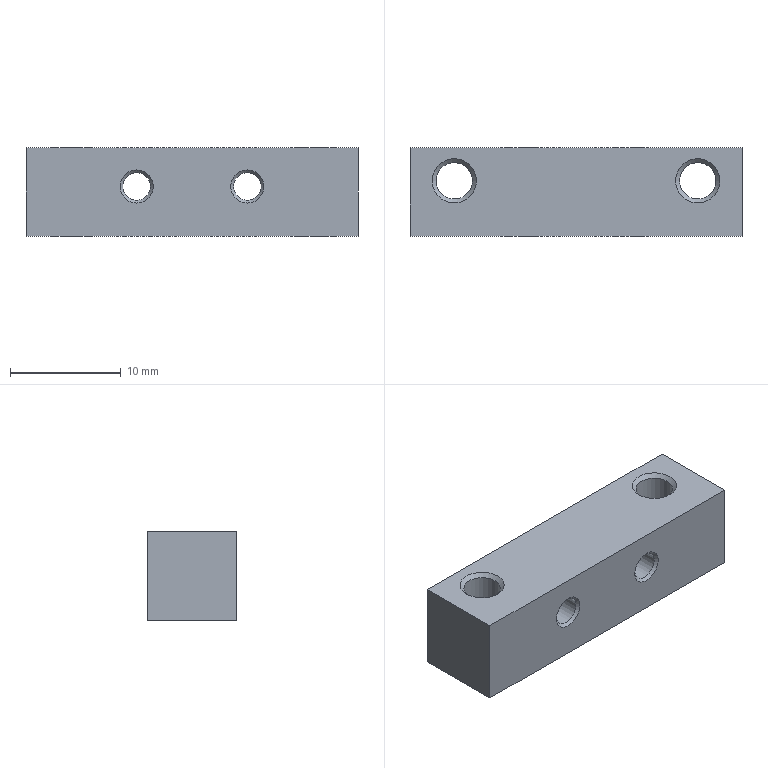Part | STEP file | Connector mounting block | 1 solid | 18 faces | box 30 x 8 x 8 mm | volume 1701 mm3 | cone 8 | plane 6 | cylinder 4 | commonest cylinder face diameters 2.5 x2 3.3 x2
STEP:
#1=CARTESIAN_POINT('',(0.,0.,0.));
#2=DIRECTION('',(0.,0.,1.));
#3=DIRECTION('',(1.,0.,0.));
#4=AXIS2_PLACEMENT_3D('',#1,#2,#3);
#5=CARTESIAN_POINT('',(-15.,4.,0.));
#6=VERTEX_POINT('',#5);
#7=CARTESIAN_POINT('',(-15.,-4.,0.));
#8=VERTEX_POINT('',#7);
#9=CARTESIAN_POINT('',(-15.,4.,0.));
#10=DIRECTION('',(0.,-1.,0.));
#11=VECTOR('',#10,1.);
#12=LINE('',#9,#11);
#13=CARTESIAN_POINT('',(-15.,4.,4.));
#14=DIRECTION('',(1.,0.,0.));
#15=DIRECTION('',(0.,1.,0.));
#16=AXIS2_PLACEMENT_3D('',#13,#14,#15);
#17=PLANE('',#16);
#18=CARTESIAN_POINT('',(0.,-4.));
#19=DIRECTION('',(-1.,0.));
#20=VECTOR('',#19,1.);
#21=LINE('',#18,#20);
#22=(GEOMETRIC_REPRESENTATION_CONTEXT(2)PARAMETRIC_REPRESENTATION_CONTEXT()REPRESENTATION_CONTEXT('',''));
#23=DEFINITIONAL_REPRESENTATION('',(#21),#22);
#24=PCURVE('',#17,#23);
#25=CARTESIAN_POINT('',(0.,0.,0.));
#26=DIRECTION('',(0.,0.,1.));
#27=DIRECTION('',(1.,0.,0.));
#28=AXIS2_PLACEMENT_3D('',#25,#26,#27);
#29=PLANE('',#28);
#30=CARTESIAN_POINT('',(-15.,4.));
#31=DIRECTION('',(0.,-1.));
#32=VECTOR('',#31,1.);
#33=LINE('',#30,#32);
#34=(GEOMETRIC_REPRESENTATION_CONTEXT(2)PARAMETRIC_REPRESENTATION_CONTEXT()REPRESENTATION_CONTEXT('',''));
#35=DEFINITIONAL_REPRESENTATION('',(#33),#34);
#36=PCURVE('',#29,#35);
#37=SURFACE_CURVE('',#12,(#24,#36),.PCURVE_S1.);
#38=EDGE_CURVE('',#6,#8,#37,.T.);
#39=ORIENTED_EDGE('',*,*,#38,.T.);
#40=CARTESIAN_POINT('',(-15.,-4.,8.));
#41=VERTEX_POINT('',#40);
#42=CARTESIAN_POINT('',(-15.,-4.,4.));
#43=DIRECTION('',(0.,0.,-1.));
#44=VECTOR('',#43,1.);
#45=LINE('',#42,#44);
#46=CARTESIAN_POINT('',(-8.,0.));
#47=DIRECTION('',(0.,-1.));
#48=VECTOR('',#47,1.);
#49=LINE('',#46,#48);
#50=(GEOMETRIC_REPRESENTATION_CONTEXT(2)PARAMETRIC_REPRESENTATION_CONTEXT()REPRESENTATION_CONTEXT('',''));
#51=DEFINITIONAL_REPRESENTATION('',(#49),#50);
#52=PCURVE('',#17,#51);
#53=CARTESIAN_POINT('',(-15.,-4.,4.));
#54=DIRECTION('',(0.,1.,0.));
#55=DIRECTION('',(0.,0.,1.));
#56=AXIS2_PLACEMENT_3D('',#53,#54,#55);
#57=PLANE('',#56);
#58=CARTESIAN_POINT('',(0.,0.));
#59=DIRECTION('',(-1.,0.));
#60=VECTOR('',#59,1.);
#61=LINE('',#58,#60);
#62=(GEOMETRIC_REPRESENTATION_CONTEXT(2)PARAMETRIC_REPRESENTATION_CONTEXT()REPRESENTATION_CONTEXT('',''));
#63=DEFINITIONAL_REPRESENTATION('',(#61),#62);
#64=PCURVE('',#57,#63);
#65=SURFACE_CURVE('',#45,(#52,#64),.PCURVE_S1.);
#66=EDGE_CURVE('',#41,#8,#65,.T.);
#67=ORIENTED_EDGE('',*,*,#66,.F.);
#68=CARTESIAN_POINT('',(-15.,4.,8.));
#69=VERTEX_POINT('',#68);
#70=CARTESIAN_POINT('',(-15.,4.,8.));
#71=DIRECTION('',(0.,-1.,0.));
#72=VECTOR('',#71,1.);
#73=LINE('',#70,#72);
#74=CARTESIAN_POINT('',(0.,4.));
#75=DIRECTION('',(-1.,0.));
#76=VECTOR('',#75,1.);
#77=LINE('',#74,#76);
#78=(GEOMETRIC_REPRESENTATION_CONTEXT(2)PARAMETRIC_REPRESENTATION_CONTEXT()REPRESENTATION_CONTEXT('',''));
#79=DEFINITIONAL_REPRESENTATION('',(#77),#78);
#80=PCURVE('',#17,#79);
#81=CARTESIAN_POINT('',(0.,0.,8.));
#82=DIRECTION('',(0.,0.,1.));
#83=DIRECTION('',(1.,0.,0.));
#84=AXIS2_PLACEMENT_3D('',#81,#82,#83);
#85=PLANE('',#84);
#86=CARTESIAN_POINT('',(-15.,4.));
#87=DIRECTION('',(0.,-1.));
#88=VECTOR('',#87,1.);
#89=LINE('',#86,#88);
#90=(GEOMETRIC_REPRESENTATION_CONTEXT(2)PARAMETRIC_REPRESENTATION_CONTEXT()REPRESENTATION_CONTEXT('',''));
#91=DEFINITIONAL_REPRESENTATION('',(#89),#90);
#92=PCURVE('',#85,#91);
#93=SURFACE_CURVE('',#73,(#80,#92),.PCURVE_S1.);
#94=EDGE_CURVE('',#69,#41,#93,.T.);
#95=ORIENTED_EDGE('',*,*,#94,.F.);
#96=CARTESIAN_POINT('',(-15.,4.,4.));
#97=DIRECTION('',(0.,0.,-1.));
#98=VECTOR('',#97,1.);
#99=LINE('',#96,#98);
#100=CARTESIAN_POINT('',(0.,0.));
#101=DIRECTION('',(0.,-1.));
#102=VECTOR('',#101,1.);
#103=LINE('',#100,#102);
#104=(GEOMETRIC_REPRESENTATION_CONTEXT(2)PARAMETRIC_REPRESENTATION_CONTEXT()REPRESENTATION_CONTEXT('',''));
#105=DEFINITIONAL_REPRESENTATION('',(#103),#104);
#106=PCURVE('',#17,#105);
#107=CARTESIAN_POINT('',(15.,4.,4.));
#108=DIRECTION('',(0.,-1.,0.));
#109=DIRECTION('',(0.,0.,-1.));
#110=AXIS2_PLACEMENT_3D('',#107,#108,#109);
#111=PLANE('',#110);
#112=CARTESIAN_POINT('',(0.,-30.));
#113=DIRECTION('',(1.,0.));
#114=VECTOR('',#113,1.);
#115=LINE('',#112,#114);
#116=(GEOMETRIC_REPRESENTATION_CONTEXT(2)PARAMETRIC_REPRESENTATION_CONTEXT()REPRESENTATION_CONTEXT('',''));
#117=DEFINITIONAL_REPRESENTATION('',(#115),#116);
#118=PCURVE('',#111,#117);
#119=SURFACE_CURVE('',#99,(#106,#118),.PCURVE_S1.);
#120=EDGE_CURVE('',#69,#6,#119,.T.);
#121=ORIENTED_EDGE('',*,*,#120,.T.);
#122=EDGE_LOOP('',(#39,#67,#95,#121));
#123=FACE_BOUND('',#122,.T.);
#124=ADVANCED_FACE('',(#123),#17,.F.);
#125=CARTESIAN_POINT('',(5.,-4.,6.));
#126=VERTEX_POINT('',#125);
#127=CARTESIAN_POINT('',(5.,-4.,4.5));
#128=DIRECTION('',(0.,1.,0.));
#129=DIRECTION('',(0.,0.,1.));
#130=AXIS2_PLACEMENT_3D('',#127,#128,#129);
#131=CIRCLE('',#130,1.5);
#132=CARTESIAN_POINT('',(0.5,20.));
#133=DIRECTION('',(1.,0.));
#134=AXIS2_PLACEMENT_2D('',#132,#133);
#135=CIRCLE('',#134,1.5);
#136=(GEOMETRIC_REPRESENTATION_CONTEXT(2)PARAMETRIC_REPRESENTATION_CONTEXT()REPRESENTATION_CONTEXT('',''));
#137=DEFINITIONAL_REPRESENTATION('',(#135),#136);
#138=PCURVE('',#57,#137);
#139=CARTESIAN_POINT('',(5.,-2.5,4.5));
#140=DIRECTION('',(0.,-1.,0.));
#141=DIRECTION('',(-1.,0.,0.));
#142=AXIS2_PLACEMENT_3D('',#139,#140,#141);
#143=CONICAL_SURFACE('',#142,0.,0.7854);
#144=CARTESIAN_POINT('',(10.996,1.5));
#145=DIRECTION('',(-1.,0.));
#146=VECTOR('',#145,1.);
#147=LINE('',#144,#146);
#148=(GEOMETRIC_REPRESENTATION_CONTEXT(2)PARAMETRIC_REPRESENTATION_CONTEXT()REPRESENTATION_CONTEXT('',''));
#149=DEFINITIONAL_REPRESENTATION('',(#147),#148);
#150=PCURVE('',#143,#149);
#151=SURFACE_CURVE('',#131,(#138,#150),.PCURVE_S1.);
#152=EDGE_CURVE('',#126,#126,#151,.T.);
#153=ORIENTED_EDGE('',*,*,#152,.T.);
#154=EDGE_LOOP('',(#153));
#155=FACE_BOUND('',#154,.T.);
#156=CARTESIAN_POINT('',(-5.,-4.,6.));
#157=VERTEX_POINT('',#156);
#158=CARTESIAN_POINT('',(-5.,-4.,4.5));
#159=DIRECTION('',(0.,1.,0.));
#160=DIRECTION('',(0.,0.,1.));
#161=AXIS2_PLACEMENT_3D('',#158,#159,#160);
#162=CIRCLE('',#161,1.5);
#163=CARTESIAN_POINT('',(0.5,10.));
#164=DIRECTION('',(1.,0.));
#165=AXIS2_PLACEMENT_2D('',#163,#164);
#166=CIRCLE('',#165,1.5);
#167=(GEOMETRIC_REPRESENTATION_CONTEXT(2)PARAMETRIC_REPRESENTATION_CONTEXT()REPRESENTATION_CONTEXT('',''));
#168=DEFINITIONAL_REPRESENTATION('',(#166),#167);
#169=PCURVE('',#57,#168);
#170=CARTESIAN_POINT('',(-5.,-2.5,4.5));
#171=DIRECTION('',(0.,-1.,0.));
#172=DIRECTION('',(-1.,0.,0.));
#173=AXIS2_PLACEMENT_3D('',#170,#171,#172);
#174=CONICAL_SURFACE('',#173,0.,0.7854);
#175=CARTESIAN_POINT('',(10.996,1.5));
#176=DIRECTION('',(-1.,0.));
#177=VECTOR('',#176,1.);
#178=LINE('',#175,#177);
#179=(GEOMETRIC_REPRESENTATION_CONTEXT(2)PARAMETRIC_REPRESENTATION_CONTEXT()REPRESENTATION_CONTEXT('',''));
#180=DEFINITIONAL_REPRESENTATION('',(#178),#179);
#181=PCURVE('',#174,#180);
#182=SURFACE_CURVE('',#162,(#169,#181),.PCURVE_S1.);
#183=EDGE_CURVE('',#157,#157,#182,.T.);
#184=ORIENTED_EDGE('',*,*,#183,.T.);
#185=EDGE_LOOP('',(#184));
#186=FACE_BOUND('',#185,.T.);
#187=ORIENTED_EDGE('',*,*,#66,.T.);
#188=CARTESIAN_POINT('',(15.,-4.,0.));
#189=VERTEX_POINT('',#188);
#190=CARTESIAN_POINT('',(-15.,-4.,0.));
#191=DIRECTION('',(1.,0.,0.));
#192=VECTOR('',#191,1.);
#193=LINE('',#190,#192);
#194=CARTESIAN_POINT('',(-4.,0.));
#195=DIRECTION('',(0.,1.));
#196=VECTOR('',#195,1.);
#197=LINE('',#194,#196);
#198=(GEOMETRIC_REPRESENTATION_CONTEXT(2)PARAMETRIC_REPRESENTATION_CONTEXT()REPRESENTATION_CONTEXT('',''));
#199=DEFINITIONAL_REPRESENTATION('',(#197),#198);
#200=PCURVE('',#57,#199);
#201=CARTESIAN_POINT('',(-15.,-4.));
#202=DIRECTION('',(1.,0.));
#203=VECTOR('',#202,1.);
#204=LINE('',#201,#203);
#205=(GEOMETRIC_REPRESENTATION_CONTEXT(2)PARAMETRIC_REPRESENTATION_CONTEXT()REPRESENTATION_CONTEXT('',''));
#206=DEFINITIONAL_REPRESENTATION('',(#204),#205);
#207=PCURVE('',#29,#206);
#208=SURFACE_CURVE('',#193,(#200,#207),.PCURVE_S1.);
#209=EDGE_CURVE('',#8,#189,#208,.T.);
#210=ORIENTED_EDGE('',*,*,#209,.T.);
#211=CARTESIAN_POINT('',(15.,-4.,8.));
#212=VERTEX_POINT('',#211);
#213=CARTESIAN_POINT('',(15.,-4.,4.));
#214=DIRECTION('',(0.,0.,-1.));
#215=VECTOR('',#214,1.);
#216=LINE('',#213,#215);
#217=CARTESIAN_POINT('',(0.,30.));
#218=DIRECTION('',(-1.,0.));
#219=VECTOR('',#218,1.);
#220=LINE('',#217,#219);
#221=(GEOMETRIC_REPRESENTATION_CONTEXT(2)PARAMETRIC_REPRESENTATION_CONTEXT()REPRESENTATION_CONTEXT('',''));
#222=DEFINITIONAL_REPRESENTATION('',(#220),#221);
#223=PCURVE('',#57,#222);
#224=CARTESIAN_POINT('',(15.,-4.,4.));
#225=DIRECTION('',(-1.,0.,0.));
#226=DIRECTION('',(0.,-1.,0.));
#227=AXIS2_PLACEMENT_3D('',#224,#225,#226);
#228=PLANE('',#227);
#229=CARTESIAN_POINT('',(0.,0.));
#230=DIRECTION('',(0.,-1.));
#231=VECTOR('',#230,1.);
#232=LINE('',#229,#231);
#233=(GEOMETRIC_REPRESENTATION_CONTEXT(2)PARAMETRIC_REPRESENTATION_CONTEXT()REPRESENTATION_CONTEXT('',''));
#234=DEFINITIONAL_REPRESENTATION('',(#232),#233);
#235=PCURVE('',#228,#234);
#236=SURFACE_CURVE('',#216,(#223,#235),.PCURVE_S1.);
#237=EDGE_CURVE('',#212,#189,#236,.T.);
#238=ORIENTED_EDGE('',*,*,#237,.F.);
#239=CARTESIAN_POINT('',(-15.,-4.,8.));
#240=DIRECTION('',(1.,0.,0.));
#241=VECTOR('',#240,1.);
#242=LINE('',#239,#241);
#243=CARTESIAN_POINT('',(4.,0.));
#244=DIRECTION('',(0.,1.));
#245=VECTOR('',#244,1.);
#246=LINE('',#243,#245);
#247=(GEOMETRIC_REPRESENTATION_CONTEXT(2)PARAMETRIC_REPRESENTATION_CONTEXT()REPRESENTATION_CONTEXT('',''));
#248=DEFINITIONAL_REPRESENTATION('',(#246),#247);
#249=PCURVE('',#57,#248);
#250=CARTESIAN_POINT('',(-15.,-4.));
#251=DIRECTION('',(1.,0.));
#252=VECTOR('',#251,1.);
#253=LINE('',#250,#252);
#254=(GEOMETRIC_REPRESENTATION_CONTEXT(2)PARAMETRIC_REPRESENTATION_CONTEXT()REPRESENTATION_CONTEXT('',''));
#255=DEFINITIONAL_REPRESENTATION('',(#253),#254);
#256=PCURVE('',#85,#255);
#257=SURFACE_CURVE('',#242,(#249,#256),.PCURVE_S1.);
#258=EDGE_CURVE('',#41,#212,#257,.T.);
#259=ORIENTED_EDGE('',*,*,#258,.F.);
#260=EDGE_LOOP('',(#187,#210,#238,#259));
#261=FACE_BOUND('',#260,.T.);
#262=ADVANCED_FACE('',(#155,#186,#261),#57,.F.);
#263=CARTESIAN_POINT('',(15.,4.,0.));
#264=VERTEX_POINT('',#263);
#265=CARTESIAN_POINT('',(15.,-4.,0.));
#266=DIRECTION('',(0.,1.,0.));
#267=VECTOR('',#266,1.);
#268=LINE('',#265,#267);
#269=CARTESIAN_POINT('',(0.,-4.));
#270=DIRECTION('',(-1.,0.));
#271=VECTOR('',#270,1.);
#272=LINE('',#269,#271);
#273=(GEOMETRIC_REPRESENTATION_CONTEXT(2)PARAMETRIC_REPRESENTATION_CONTEXT()REPRESENTATION_CONTEXT('',''));
#274=DEFINITIONAL_REPRESENTATION('',(#272),#273);
#275=PCURVE('',#228,#274);
#276=CARTESIAN_POINT('',(15.,-4.));
#277=DIRECTION('',(0.,1.));
#278=VECTOR('',#277,1.);
#279=LINE('',#276,#278);
#280=(GEOMETRIC_REPRESENTATION_CONTEXT(2)PARAMETRIC_REPRESENTATION_CONTEXT()REPRESENTATION_CONTEXT('',''));
#281=DEFINITIONAL_REPRESENTATION('',(#279),#280);
#282=PCURVE('',#29,#281);
#283=SURFACE_CURVE('',#268,(#275,#282),.PCURVE_S1.);
#284=EDGE_CURVE('',#189,#264,#283,.T.);
#285=ORIENTED_EDGE('',*,*,#284,.T.);
#286=CARTESIAN_POINT('',(15.,4.,8.));
#287=VERTEX_POINT('',#286);
#288=CARTESIAN_POINT('',(15.,4.,4.));
#289=DIRECTION('',(0.,0.,-1.));
#290=VECTOR('',#289,1.);
#291=LINE('',#288,#290);
#292=CARTESIAN_POINT('',(-8.,0.));
#293=DIRECTION('',(0.,-1.));
#294=VECTOR('',#293,1.);
#295=LINE('',#292,#294);
#296=(GEOMETRIC_REPRESENTATION_CONTEXT(2)PARAMETRIC_REPRESENTATION_CONTEXT()REPRESENTATION_CONTEXT('',''));
#297=DEFINITIONAL_REPRESENTATION('',(#295),#296);
#298=PCURVE('',#228,#297);
#299=CARTESIAN_POINT('',(0.,0.));
#300=DIRECTION('',(1.,0.));
#301=VECTOR('',#300,1.);
#302=LINE('',#299,#301);
#303=(GEOMETRIC_REPRESENTATION_CONTEXT(2)PARAMETRIC_REPRESENTATION_CONTEXT()REPRESENTATION_CONTEXT('',''));
#304=DEFINITIONAL_REPRESENTATION('',(#302),#303);
#305=PCURVE('',#111,#304);
#306=SURFACE_CURVE('',#291,(#298,#305),.PCURVE_S1.);
#307=EDGE_CURVE('',#287,#264,#306,.T.);
#308=ORIENTED_EDGE('',*,*,#307,.F.);
#309=CARTESIAN_POINT('',(15.,-4.,8.));
#310=DIRECTION('',(0.,1.,0.));
#311=VECTOR('',#310,1.);
#312=LINE('',#309,#311);
#313=CARTESIAN_POINT('',(0.,4.));
#314=DIRECTION('',(-1.,0.));
#315=VECTOR('',#314,1.);
#316=LINE('',#313,#315);
#317=(GEOMETRIC_REPRESENTATION_CONTEXT(2)PARAMETRIC_REPRESENTATION_CONTEXT()REPRESENTATION_CONTEXT('',''));
#318=DEFINITIONAL_REPRESENTATION('',(#316),#317);
#319=PCURVE('',#228,#318);
#320=CARTESIAN_POINT('',(15.,-4.));
#321=DIRECTION('',(0.,1.));
#322=VECTOR('',#321,1.);
#323=LINE('',#320,#322);
#324=(GEOMETRIC_REPRESENTATION_CONTEXT(2)PARAMETRIC_REPRESENTATION_CONTEXT()REPRESENTATION_CONTEXT('',''));
#325=DEFINITIONAL_REPRESENTATION('',(#323),#324);
#326=PCURVE('',#85,#325);
#327=SURFACE_CURVE('',#312,(#319,#326),.PCURVE_S1.);
#328=EDGE_CURVE('',#212,#287,#327,.T.);
#329=ORIENTED_EDGE('',*,*,#328,.F.);
#330=ORIENTED_EDGE('',*,*,#237,.T.);
#331=EDGE_LOOP('',(#285,#308,#329,#330));
#332=FACE_BOUND('',#331,.T.);
#333=ADVANCED_FACE('',(#332),#228,.F.);
#334=CARTESIAN_POINT('',(5.,4.,3.));
#335=VERTEX_POINT('',#334);
#336=CARTESIAN_POINT('',(5.,4.,4.5));
#337=DIRECTION('',(0.,-1.,0.));
#338=DIRECTION('',(0.,0.,-1.));
#339=AXIS2_PLACEMENT_3D('',#336,#337,#338);
#340=CIRCLE('',#339,1.5);
#341=CARTESIAN_POINT('',(-0.5,-10.));
#342=DIRECTION('',(1.,0.));
#343=AXIS2_PLACEMENT_2D('',#341,#342);
#344=CIRCLE('',#343,1.5);
#345=(GEOMETRIC_REPRESENTATION_CONTEXT(2)PARAMETRIC_REPRESENTATION_CONTEXT()REPRESENTATION_CONTEXT('',''));
#346=DEFINITIONAL_REPRESENTATION('',(#344),#345);
#347=PCURVE('',#111,#346);
#348=CARTESIAN_POINT('',(5.,2.5,4.5));
#349=DIRECTION('',(0.,1.,0.));
#350=DIRECTION('',(1.,0.,0.));
#351=AXIS2_PLACEMENT_3D('',#348,#349,#350);
#352=CONICAL_SURFACE('',#351,0.,0.7854);
#353=CARTESIAN_POINT('',(7.854,1.5));
#354=DIRECTION('',(-1.,0.));
#355=VECTOR('',#354,1.);
#356=LINE('',#353,#355);
#357=(GEOMETRIC_REPRESENTATION_CONTEXT(2)PARAMETRIC_REPRESENTATION_CONTEXT()REPRESENTATION_CONTEXT('',''));
#358=DEFINITIONAL_REPRESENTATION('',(#356),#357);
#359=PCURVE('',#352,#358);
#360=SURFACE_CURVE('',#340,(#347,#359),.PCURVE_S1.);
#361=EDGE_CURVE('',#335,#335,#360,.T.);
#362=ORIENTED_EDGE('',*,*,#361,.T.);
#363=EDGE_LOOP('',(#362));
#364=FACE_BOUND('',#363,.T.);
#365=CARTESIAN_POINT('',(-5.,4.,3.));
#366=VERTEX_POINT('',#365);
#367=CARTESIAN_POINT('',(-5.,4.,6.));
#368=VERTEX_POINT('',#367);
#369=CARTESIAN_POINT('',(-5.,4.,4.5));
#370=DIRECTION('',(0.,-1.,0.));
#371=DIRECTION('',(0.,0.,-1.));
#372=AXIS2_PLACEMENT_3D('',#369,#370,#371);
#373=CIRCLE('',#372,1.5);
#374=CARTESIAN_POINT('',(-0.5,-20.));
#375=DIRECTION('',(1.,0.));
#376=AXIS2_PLACEMENT_2D('',#374,#375);
#377=CIRCLE('',#376,1.5);
#378=(GEOMETRIC_REPRESENTATION_CONTEXT(2)PARAMETRIC_REPRESENTATION_CONTEXT()REPRESENTATION_CONTEXT('',''));
#379=DEFINITIONAL_REPRESENTATION('',(#377),#378);
#380=PCURVE('',#111,#379);
#381=CARTESIAN_POINT('',(-5.,2.5,4.5));
#382=DIRECTION('',(0.,1.,0.));
#383=DIRECTION('',(1.,0.,0.));
#384=AXIS2_PLACEMENT_3D('',#381,#382,#383);
#385=CONICAL_SURFACE('',#384,0.,0.7854);
#386=CARTESIAN_POINT('',(7.854,1.5));
#387=DIRECTION('',(-1.,0.));
#388=VECTOR('',#387,1.);
#389=LINE('',#386,#388);
#390=(GEOMETRIC_REPRESENTATION_CONTEXT(2)PARAMETRIC_REPRESENTATION_CONTEXT()REPRESENTATION_CONTEXT('',''));
#391=DEFINITIONAL_REPRESENTATION('',(#389),#390);
#392=PCURVE('',#385,#391);
#393=SURFACE_CURVE('',#373,(#380,#392),.PCURVE_S1.);
#394=EDGE_CURVE('',#366,#368,#393,.T.);
#395=ORIENTED_EDGE('',*,*,#394,.T.);
#396=CARTESIAN_POINT('',(-5.,4.,4.5));
#397=DIRECTION('',(0.,-1.,0.));
#398=DIRECTION('',(0.,0.,-1.));
#399=AXIS2_PLACEMENT_3D('',#396,#397,#398);
#400=CIRCLE('',#399,1.5);
#401=CARTESIAN_POINT('',(-0.5,-20.));
#402=DIRECTION('',(1.,0.));
#403=AXIS2_PLACEMENT_2D('',#401,#402);
#404=CIRCLE('',#403,1.5);
#405=(GEOMETRIC_REPRESENTATION_CONTEXT(2)PARAMETRIC_REPRESENTATION_CONTEXT()REPRESENTATION_CONTEXT('',''));
#406=DEFINITIONAL_REPRESENTATION('',(#404),#405);
#407=PCURVE('',#111,#406);
#408=CARTESIAN_POINT('',(14.137,1.5));
#409=DIRECTION('',(-1.,0.));
#410=VECTOR('',#409,1.);
#411=LINE('',#408,#410);
#412=(GEOMETRIC_REPRESENTATION_CONTEXT(2)PARAMETRIC_REPRESENTATION_CONTEXT()REPRESENTATION_CONTEXT('',''));
#413=DEFINITIONAL_REPRESENTATION('',(#411),#412);
#414=PCURVE('',#385,#413);
#415=SURFACE_CURVE('',#400,(#407,#414),.PCURVE_S1.);
#416=EDGE_CURVE('',#368,#366,#415,.T.);
#417=ORIENTED_EDGE('',*,*,#416,.T.);
#418=EDGE_LOOP('',(#395,#417));
#419=FACE_BOUND('',#418,.T.);
#420=CARTESIAN_POINT('',(15.,4.,0.));
#421=DIRECTION('',(-1.,0.,0.));
#422=VECTOR('',#421,1.);
#423=LINE('',#420,#422);
#424=CARTESIAN_POINT('',(4.,0.));
#425=DIRECTION('',(0.,-1.));
#426=VECTOR('',#425,1.);
#427=LINE('',#424,#426);
#428=(GEOMETRIC_REPRESENTATION_CONTEXT(2)PARAMETRIC_REPRESENTATION_CONTEXT()REPRESENTATION_CONTEXT('',''));
#429=DEFINITIONAL_REPRESENTATION('',(#427),#428);
#430=PCURVE('',#111,#429);
#431=CARTESIAN_POINT('',(15.,4.));
#432=DIRECTION('',(-1.,0.));
#433=VECTOR('',#432,1.);
#434=LINE('',#431,#433);
#435=(GEOMETRIC_REPRESENTATION_CONTEXT(2)PARAMETRIC_REPRESENTATION_CONTEXT()REPRESENTATION_CONTEXT('',''));
#436=DEFINITIONAL_REPRESENTATION('',(#434),#435);
#437=PCURVE('',#29,#436);
#438=SURFACE_CURVE('',#423,(#430,#437),.PCURVE_S1.);
#439=EDGE_CURVE('',#264,#6,#438,.T.);
#440=ORIENTED_EDGE('',*,*,#439,.T.);
#441=ORIENTED_EDGE('',*,*,#120,.F.);
#442=CARTESIAN_POINT('',(15.,4.,8.));
#443=DIRECTION('',(-1.,0.,0.));
#444=VECTOR('',#443,1.);
#445=LINE('',#442,#444);
#446=CARTESIAN_POINT('',(-4.,0.));
#447=DIRECTION('',(0.,-1.));
#448=VECTOR('',#447,1.);
#449=LINE('',#446,#448);
#450=(GEOMETRIC_REPRESENTATION_CONTEXT(2)PARAMETRIC_REPRESENTATION_CONTEXT()REPRESENTATION_CONTEXT('',''));
#451=DEFINITIONAL_REPRESENTATION('',(#449),#450);
#452=PCURVE('',#111,#451);
#453=CARTESIAN_POINT('',(15.,4.));
#454=DIRECTION('',(-1.,0.));
#455=VECTOR('',#454,1.);
#456=LINE('',#453,#455);
#457=(GEOMETRIC_REPRESENTATION_CONTEXT(2)PARAMETRIC_REPRESENTATION_CONTEXT()REPRESENTATION_CONTEXT('',''));
#458=DEFINITIONAL_REPRESENTATION('',(#456),#457);
#459=PCURVE('',#85,#458);
#460=SURFACE_CURVE('',#445,(#452,#459),.PCURVE_S1.);
#461=EDGE_CURVE('',#287,#69,#460,.T.);
#462=ORIENTED_EDGE('',*,*,#461,.F.);
#463=ORIENTED_EDGE('',*,*,#307,.T.);
#464=EDGE_LOOP('',(#440,#441,#462,#463));
#465=FACE_BOUND('',#464,.T.);
#466=ADVANCED_FACE('',(#364,#419,#465),#111,.F.);
#467=ORIENTED_EDGE('',*,*,#209,.F.);
#468=ORIENTED_EDGE('',*,*,#38,.F.);
#469=ORIENTED_EDGE('',*,*,#439,.F.);
#470=ORIENTED_EDGE('',*,*,#284,.F.);
#471=EDGE_LOOP('',(#467,#468,#469,#470));
#472=FACE_BOUND('',#471,.T.);
#473=CARTESIAN_POINT('',(-9.,1.,0.));
#474=VERTEX_POINT('',#473);
#475=CARTESIAN_POINT('',(-11.,1.,0.));
#476=DIRECTION('',(0.,0.,1.));
#477=DIRECTION('',(1.,0.,0.));
#478=AXIS2_PLACEMENT_3D('',#475,#476,#477);
#479=CIRCLE('',#478,2.);
#480=CARTESIAN_POINT('',(-11.,1.));
#481=DIRECTION('',(1.,0.));
#482=AXIS2_PLACEMENT_2D('',#480,#481);
#483=CIRCLE('',#482,2.);
#484=(GEOMETRIC_REPRESENTATION_CONTEXT(2)PARAMETRIC_REPRESENTATION_CONTEXT()REPRESENTATION_CONTEXT('',''));
#485=DEFINITIONAL_REPRESENTATION('',(#483),#484);
#486=PCURVE('',#29,#485);
#487=CARTESIAN_POINT('',(-11.,1.,2.));
#488=DIRECTION('',(0.,0.,-1.));
#489=DIRECTION('',(-1.,0.,0.));
#490=AXIS2_PLACEMENT_3D('',#487,#488,#489);
#491=CONICAL_SURFACE('',#490,0.,0.7854);
#492=CARTESIAN_POINT('',(9.425,2.));
#493=DIRECTION('',(-1.,0.));
#494=VECTOR('',#493,1.);
#495=LINE('',#492,#494);
#496=(GEOMETRIC_REPRESENTATION_CONTEXT(2)PARAMETRIC_REPRESENTATION_CONTEXT()REPRESENTATION_CONTEXT('',''));
#497=DEFINITIONAL_REPRESENTATION('',(#495),#496);
#498=PCURVE('',#491,#497);
#499=SURFACE_CURVE('',#479,(#486,#498),.PCURVE_S1.);
#500=EDGE_CURVE('',#474,#474,#499,.T.);
#501=ORIENTED_EDGE('',*,*,#500,.T.);
#502=EDGE_LOOP('',(#501));
#503=FACE_BOUND('',#502,.T.);
#504=CARTESIAN_POINT('',(13.,1.,0.));
#505=VERTEX_POINT('',#504);
#506=CARTESIAN_POINT('',(11.,1.,0.));
#507=DIRECTION('',(0.,0.,1.));
#508=DIRECTION('',(1.,0.,0.));
#509=AXIS2_PLACEMENT_3D('',#506,#507,#508);
#510=CIRCLE('',#509,2.);
#511=CARTESIAN_POINT('',(11.,1.));
#512=DIRECTION('',(1.,0.));
#513=AXIS2_PLACEMENT_2D('',#511,#512);
#514=CIRCLE('',#513,2.);
#515=(GEOMETRIC_REPRESENTATION_CONTEXT(2)PARAMETRIC_REPRESENTATION_CONTEXT()REPRESENTATION_CONTEXT('',''));
#516=DEFINITIONAL_REPRESENTATION('',(#514),#515);
#517=PCURVE('',#29,#516);
#518=CARTESIAN_POINT('',(11.,1.,2.));
#519=DIRECTION('',(0.,0.,-1.));
#520=DIRECTION('',(-1.,0.,0.));
#521=AXIS2_PLACEMENT_3D('',#518,#519,#520);
#522=CONICAL_SURFACE('',#521,0.,0.7854);
#523=CARTESIAN_POINT('',(9.425,2.));
#524=DIRECTION('',(-1.,0.));
#525=VECTOR('',#524,1.);
#526=LINE('',#523,#525);
#527=(GEOMETRIC_REPRESENTATION_CONTEXT(2)PARAMETRIC_REPRESENTATION_CONTEXT()REPRESENTATION_CONTEXT('',''));
#528=DEFINITIONAL_REPRESENTATION('',(#526),#527);
#529=PCURVE('',#522,#528);
#530=SURFACE_CURVE('',#510,(#517,#529),.PCURVE_S1.);
#531=EDGE_CURVE('',#505,#505,#530,.T.);
#532=ORIENTED_EDGE('',*,*,#531,.T.);
#533=EDGE_LOOP('',(#532));
#534=FACE_BOUND('',#533,.T.);
#535=ADVANCED_FACE('',(#472,#503,#534),#29,.F.);
#536=CARTESIAN_POINT('',(13.,1.,8.));
#537=VERTEX_POINT('',#536);
#538=CARTESIAN_POINT('',(11.,1.,8.));
#539=DIRECTION('',(0.,0.,1.));
#540=DIRECTION('',(1.,0.,0.));
#541=AXIS2_PLACEMENT_3D('',#538,#539,#540);
#542=CIRCLE('',#541,2.);
#543=CARTESIAN_POINT('',(11.,1.));
#544=DIRECTION('',(1.,0.));
#545=AXIS2_PLACEMENT_2D('',#543,#544);
#546=CIRCLE('',#545,2.);
#547=(GEOMETRIC_REPRESENTATION_CONTEXT(2)PARAMETRIC_REPRESENTATION_CONTEXT()REPRESENTATION_CONTEXT('',''));
#548=DEFINITIONAL_REPRESENTATION('',(#546),#547);
#549=PCURVE('',#85,#548);
#550=CARTESIAN_POINT('',(11.,1.,6.));
#551=DIRECTION('',(0.,0.,1.));
#552=DIRECTION('',(1.,0.,0.));
#553=AXIS2_PLACEMENT_3D('',#550,#551,#552);
#554=CONICAL_SURFACE('',#553,0.,0.7854);
#555=CARTESIAN_POINT('',(0.,2.));
#556=DIRECTION('',(1.,0.));
#557=VECTOR('',#556,1.);
#558=LINE('',#555,#557);
#559=(GEOMETRIC_REPRESENTATION_CONTEXT(2)PARAMETRIC_REPRESENTATION_CONTEXT()REPRESENTATION_CONTEXT('',''));
#560=DEFINITIONAL_REPRESENTATION('',(#558),#559);
#561=PCURVE('',#554,#560);
#562=SURFACE_CURVE('',#542,(#549,#561),.PCURVE_S1.);
#563=EDGE_CURVE('',#537,#537,#562,.T.);
#564=ORIENTED_EDGE('',*,*,#563,.F.);
#565=EDGE_LOOP('',(#564));
#566=FACE_BOUND('',#565,.T.);
#567=CARTESIAN_POINT('',(-9.,1.,8.));
#568=VERTEX_POINT('',#567);
#569=CARTESIAN_POINT('',(-11.,1.,8.));
#570=DIRECTION('',(0.,0.,1.));
#571=DIRECTION('',(1.,0.,0.));
#572=AXIS2_PLACEMENT_3D('',#569,#570,#571);
#573=CIRCLE('',#572,2.);
#574=CARTESIAN_POINT('',(-11.,1.));
#575=DIRECTION('',(1.,0.));
#576=AXIS2_PLACEMENT_2D('',#574,#575);
#577=CIRCLE('',#576,2.);
#578=(GEOMETRIC_REPRESENTATION_CONTEXT(2)PARAMETRIC_REPRESENTATION_CONTEXT()REPRESENTATION_CONTEXT('',''));
#579=DEFINITIONAL_REPRESENTATION('',(#577),#578);
#580=PCURVE('',#85,#579);
#581=CARTESIAN_POINT('',(-11.,1.,6.));
#582=DIRECTION('',(0.,0.,1.));
#583=DIRECTION('',(1.,0.,0.));
#584=AXIS2_PLACEMENT_3D('',#581,#582,#583);
#585=CONICAL_SURFACE('',#584,0.,0.7854);
#586=CARTESIAN_POINT('',(0.,2.));
#587=DIRECTION('',(1.,0.));
#588=VECTOR('',#587,1.);
#589=LINE('',#586,#588);
#590=(GEOMETRIC_REPRESENTATION_CONTEXT(2)PARAMETRIC_REPRESENTATION_CONTEXT()REPRESENTATION_CONTEXT('',''));
#591=DEFINITIONAL_REPRESENTATION('',(#589),#590);
#592=PCURVE('',#585,#591);
#593=SURFACE_CURVE('',#573,(#580,#592),.PCURVE_S1.);
#594=EDGE_CURVE('',#568,#568,#593,.T.);
#595=ORIENTED_EDGE('',*,*,#594,.F.);
#596=EDGE_LOOP('',(#595));
#597=FACE_BOUND('',#596,.T.);
#598=ORIENTED_EDGE('',*,*,#94,.T.);
#599=ORIENTED_EDGE('',*,*,#258,.T.);
#600=ORIENTED_EDGE('',*,*,#328,.T.);
#601=ORIENTED_EDGE('',*,*,#461,.T.);
#602=EDGE_LOOP('',(#598,#599,#600,#601));
#603=FACE_BOUND('',#602,.T.);
#604=ADVANCED_FACE('',(#566,#597,#603),#85,.T.);
#605=CARTESIAN_POINT('',(-9.35,1.,7.65));
#606=VERTEX_POINT('',#605);
#607=CARTESIAN_POINT('',(-11.,1.,7.65));
#608=DIRECTION('',(0.,0.,1.));
#609=DIRECTION('',(1.,0.,0.));
#610=AXIS2_PLACEMENT_3D('',#607,#608,#609);
#611=CIRCLE('',#610,1.65);
#612=CARTESIAN_POINT('',(-11.,1.,0.));
#613=DIRECTION('',(0.,0.,1.));
#614=DIRECTION('',(1.,0.,0.));
#615=AXIS2_PLACEMENT_3D('',#612,#613,#614);
#616=CYLINDRICAL_SURFACE('',#615,1.65);
#617=CARTESIAN_POINT('',(0.,7.65));
#618=DIRECTION('',(1.,0.));
#619=VECTOR('',#618,1.);
#620=LINE('',#617,#619);
#621=(GEOMETRIC_REPRESENTATION_CONTEXT(2)PARAMETRIC_REPRESENTATION_CONTEXT()REPRESENTATION_CONTEXT('',''));
#622=DEFINITIONAL_REPRESENTATION('',(#620),#621);
#623=PCURVE('',#616,#622);
#624=CARTESIAN_POINT('',(0.,1.65));
#625=DIRECTION('',(1.,0.));
#626=VECTOR('',#625,1.);
#627=LINE('',#624,#626);
#628=(GEOMETRIC_REPRESENTATION_CONTEXT(2)PARAMETRIC_REPRESENTATION_CONTEXT()REPRESENTATION_CONTEXT('',''));
#629=DEFINITIONAL_REPRESENTATION('',(#627),#628);
#630=PCURVE('',#585,#629);
#631=SURFACE_CURVE('',#611,(#623,#630),.PCURVE_S1.);
#632=EDGE_CURVE('',#606,#606,#631,.T.);
#633=ORIENTED_EDGE('',*,*,#632,.F.);
#634=CARTESIAN_POINT('',(-9.35,1.,0.35));
#635=VERTEX_POINT('',#634);
#636=CARTESIAN_POINT('',(-9.35,1.,0.35));
#637=CARTESIAN_POINT('',(-9.35,1.,7.65));
#638=B_SPLINE_CURVE_WITH_KNOTS('',1,(#636,#637),.UNSPECIFIED.,.F.,.F.,(2,2),(0.35,7.65),.PIECEWISE_BEZIER_KNOTS.);
#639=CARTESIAN_POINT('',(0.,0.));
#640=DIRECTION('',(0.,1.));
#641=VECTOR('',#640,1.);
#642=LINE('',#639,#641);
#643=(GEOMETRIC_REPRESENTATION_CONTEXT(2)PARAMETRIC_REPRESENTATION_CONTEXT()REPRESENTATION_CONTEXT('',''));
#644=DEFINITIONAL_REPRESENTATION('',(#642),#643);
#645=PCURVE('',#616,#644);
#646=CARTESIAN_POINT('',(6.283,0.));
#647=DIRECTION('',(0.,1.));
#648=VECTOR('',#647,1.);
#649=LINE('',#646,#648);
#650=(GEOMETRIC_REPRESENTATION_CONTEXT(2)PARAMETRIC_REPRESENTATION_CONTEXT()REPRESENTATION_CONTEXT('',''));
#651=DEFINITIONAL_REPRESENTATION('',(#649),#650);
#652=PCURVE('',#616,#651);
#653=SEAM_CURVE('',#638,(#645,#652),.PCURVE_S1.);
#654=EDGE_CURVE('',#635,#606,#653,.T.);
#655=ORIENTED_EDGE('',*,*,#654,.F.);
#656=CARTESIAN_POINT('',(-12.65,1.,0.35));
#657=VERTEX_POINT('',#656);
#658=CARTESIAN_POINT('',(-11.,1.,0.35));
#659=DIRECTION('',(0.,0.,-1.));
#660=DIRECTION('',(-1.,0.,0.));
#661=AXIS2_PLACEMENT_3D('',#658,#659,#660);
#662=CIRCLE('',#661,1.65);
#663=CARTESIAN_POINT('',(3.142,0.35));
#664=DIRECTION('',(-1.,0.));
#665=VECTOR('',#664,1.);
#666=LINE('',#663,#665);
#667=(GEOMETRIC_REPRESENTATION_CONTEXT(2)PARAMETRIC_REPRESENTATION_CONTEXT()REPRESENTATION_CONTEXT('',''));
#668=DEFINITIONAL_REPRESENTATION('',(#666),#667);
#669=PCURVE('',#616,#668);
#670=CARTESIAN_POINT('',(6.283,1.65));
#671=DIRECTION('',(1.,0.));
#672=VECTOR('',#671,1.);
#673=LINE('',#670,#672);
#674=(GEOMETRIC_REPRESENTATION_CONTEXT(2)PARAMETRIC_REPRESENTATION_CONTEXT()REPRESENTATION_CONTEXT('',''));
#675=DEFINITIONAL_REPRESENTATION('',(#673),#674);
#676=PCURVE('',#491,#675);
#677=SURFACE_CURVE('',#662,(#669,#676),.PCURVE_S1.);
#678=EDGE_CURVE('',#657,#635,#677,.T.);
#679=ORIENTED_EDGE('',*,*,#678,.F.);
#680=CARTESIAN_POINT('',(-11.,1.,0.35));
#681=DIRECTION('',(0.,0.,-1.));
#682=DIRECTION('',(-1.,0.,0.));
#683=AXIS2_PLACEMENT_3D('',#680,#681,#682);
#684=CIRCLE('',#683,1.65);
#685=CARTESIAN_POINT('',(9.425,0.35));
#686=DIRECTION('',(-1.,0.));
#687=VECTOR('',#686,1.);
#688=LINE('',#685,#687);
#689=(GEOMETRIC_REPRESENTATION_CONTEXT(2)PARAMETRIC_REPRESENTATION_CONTEXT()REPRESENTATION_CONTEXT('',''));
#690=DEFINITIONAL_REPRESENTATION('',(#688),#689);
#691=PCURVE('',#616,#690);
#692=CARTESIAN_POINT('',(0.,1.65));
#693=DIRECTION('',(1.,0.));
#694=VECTOR('',#693,1.);
#695=LINE('',#692,#694);
#696=(GEOMETRIC_REPRESENTATION_CONTEXT(2)PARAMETRIC_REPRESENTATION_CONTEXT()REPRESENTATION_CONTEXT('',''));
#697=DEFINITIONAL_REPRESENTATION('',(#695),#696);
#698=PCURVE('',#491,#697);
#699=SURFACE_CURVE('',#684,(#691,#698),.PCURVE_S1.);
#700=EDGE_CURVE('',#635,#657,#699,.T.);
#701=ORIENTED_EDGE('',*,*,#700,.F.);
#702=ORIENTED_EDGE('',*,*,#654,.T.);
#703=EDGE_LOOP('',(#633,#655,#679,#701,#702));
#704=FACE_BOUND('',#703,.F.);
#705=ADVANCED_FACE('',(#704),#616,.F.);
#706=ORIENTED_EDGE('',*,*,#700,.T.);
#707=ORIENTED_EDGE('',*,*,#678,.T.);
#708=CARTESIAN_POINT('',(-9.35,1.,0.35));
#709=CARTESIAN_POINT('',(-9.,1.,-0.000000002));
#710=B_SPLINE_CURVE_WITH_KNOTS('',1,(#708,#709),.UNSPECIFIED.,.F.,.F.,(2,2),(2.333,2.828),.PIECEWISE_BEZIER_KNOTS.);
#711=CARTESIAN_POINT('',(9.425,0.));
#712=DIRECTION('',(0.,1.));
#713=VECTOR('',#712,1.);
#714=LINE('',#711,#713);
#715=(GEOMETRIC_REPRESENTATION_CONTEXT(2)PARAMETRIC_REPRESENTATION_CONTEXT()REPRESENTATION_CONTEXT('',''));
#716=DEFINITIONAL_REPRESENTATION('',(#714),#715);
#717=PCURVE('',#491,#716);
#718=CARTESIAN_POINT('',(3.142,0.));
#719=DIRECTION('',(0.,1.));
#720=VECTOR('',#719,1.);
#721=LINE('',#718,#720);
#722=(GEOMETRIC_REPRESENTATION_CONTEXT(2)PARAMETRIC_REPRESENTATION_CONTEXT()REPRESENTATION_CONTEXT('',''));
#723=DEFINITIONAL_REPRESENTATION('',(#721),#722);
#724=PCURVE('',#491,#723);
#725=SEAM_CURVE('',#710,(#717,#724),.PCURVE_S1.);
#726=EDGE_CURVE('',#635,#474,#725,.T.);
#727=ORIENTED_EDGE('',*,*,#726,.T.);
#728=ORIENTED_EDGE('',*,*,#500,.T.);
#729=ORIENTED_EDGE('',*,*,#726,.F.);
#730=EDGE_LOOP('',(#706,#707,#727,#728,#729));
#731=FACE_BOUND('',#730,.F.);
#732=ADVANCED_FACE('',(#731),#491,.F.);
#733=ORIENTED_EDGE('',*,*,#594,.F.);
#734=CARTESIAN_POINT('',(-9.35,1.,7.65));
#735=CARTESIAN_POINT('',(-9.,1.,8.));
#736=B_SPLINE_CURVE_WITH_KNOTS('',1,(#734,#735),.UNSPECIFIED.,.F.,.F.,(2,2),(2.333,2.828),.PIECEWISE_BEZIER_KNOTS.);
#737=CARTESIAN_POINT('',(0.,0.));
#738=DIRECTION('',(0.,1.));
#739=VECTOR('',#738,1.);
#740=LINE('',#737,#739);
#741=(GEOMETRIC_REPRESENTATION_CONTEXT(2)PARAMETRIC_REPRESENTATION_CONTEXT()REPRESENTATION_CONTEXT('',''));
#742=DEFINITIONAL_REPRESENTATION('',(#740),#741);
#743=PCURVE('',#585,#742);
#744=CARTESIAN_POINT('',(6.283,0.));
#745=DIRECTION('',(0.,1.));
#746=VECTOR('',#745,1.);
#747=LINE('',#744,#746);
#748=(GEOMETRIC_REPRESENTATION_CONTEXT(2)PARAMETRIC_REPRESENTATION_CONTEXT()REPRESENTATION_CONTEXT('',''));
#749=DEFINITIONAL_REPRESENTATION('',(#747),#748);
#750=PCURVE('',#585,#749);
#751=SEAM_CURVE('',#736,(#743,#750),.PCURVE_S1.);
#752=EDGE_CURVE('',#606,#568,#751,.T.);
#753=ORIENTED_EDGE('',*,*,#752,.F.);
#754=ORIENTED_EDGE('',*,*,#632,.T.);
#755=ORIENTED_EDGE('',*,*,#752,.T.);
#756=EDGE_LOOP('',(#733,#753,#754,#755));
#757=FACE_BOUND('',#756,.F.);
#758=ADVANCED_FACE('',(#757),#585,.F.);
#759=CARTESIAN_POINT('',(12.65,1.,7.65));
#760=VERTEX_POINT('',#759);
#761=CARTESIAN_POINT('',(11.,1.,7.65));
#762=DIRECTION('',(0.,0.,1.));
#763=DIRECTION('',(1.,0.,0.));
#764=AXIS2_PLACEMENT_3D('',#761,#762,#763);
#765=CIRCLE('',#764,1.65);
#766=CARTESIAN_POINT('',(11.,1.,0.));
#767=DIRECTION('',(0.,0.,1.));
#768=DIRECTION('',(1.,0.,0.));
#769=AXIS2_PLACEMENT_3D('',#766,#767,#768);
#770=CYLINDRICAL_SURFACE('',#769,1.65);
#771=CARTESIAN_POINT('',(0.,7.65));
#772=DIRECTION('',(1.,0.));
#773=VECTOR('',#772,1.);
#774=LINE('',#771,#773);
#775=(GEOMETRIC_REPRESENTATION_CONTEXT(2)PARAMETRIC_REPRESENTATION_CONTEXT()REPRESENTATION_CONTEXT('',''));
#776=DEFINITIONAL_REPRESENTATION('',(#774),#775);
#777=PCURVE('',#770,#776);
#778=CARTESIAN_POINT('',(0.,1.65));
#779=DIRECTION('',(1.,0.));
#780=VECTOR('',#779,1.);
#781=LINE('',#778,#780);
#782=(GEOMETRIC_REPRESENTATION_CONTEXT(2)PARAMETRIC_REPRESENTATION_CONTEXT()REPRESENTATION_CONTEXT('',''));
#783=DEFINITIONAL_REPRESENTATION('',(#781),#782);
#784=PCURVE('',#554,#783);
#785=SURFACE_CURVE('',#765,(#777,#784),.PCURVE_S1.);
#786=EDGE_CURVE('',#760,#760,#785,.T.);
#787=ORIENTED_EDGE('',*,*,#786,.F.);
#788=CARTESIAN_POINT('',(12.65,1.,0.35));
#789=VERTEX_POINT('',#788);
#790=CARTESIAN_POINT('',(12.65,1.,0.35));
#791=CARTESIAN_POINT('',(12.65,1.,7.65));
#792=B_SPLINE_CURVE_WITH_KNOTS('',1,(#790,#791),.UNSPECIFIED.,.F.,.F.,(2,2),(0.35,7.65),.PIECEWISE_BEZIER_KNOTS.);
#793=CARTESIAN_POINT('',(0.,0.));
#794=DIRECTION('',(0.,1.));
#795=VECTOR('',#794,1.);
#796=LINE('',#793,#795);
#797=(GEOMETRIC_REPRESENTATION_CONTEXT(2)PARAMETRIC_REPRESENTATION_CONTEXT()REPRESENTATION_CONTEXT('',''));
#798=DEFINITIONAL_REPRESENTATION('',(#796),#797);
#799=PCURVE('',#770,#798);
#800=CARTESIAN_POINT('',(6.283,0.));
#801=DIRECTION('',(0.,1.));
#802=VECTOR('',#801,1.);
#803=LINE('',#800,#802);
#804=(GEOMETRIC_REPRESENTATION_CONTEXT(2)PARAMETRIC_REPRESENTATION_CONTEXT()REPRESENTATION_CONTEXT('',''));
#805=DEFINITIONAL_REPRESENTATION('',(#803),#804);
#806=PCURVE('',#770,#805);
#807=SEAM_CURVE('',#792,(#799,#806),.PCURVE_S1.);
#808=EDGE_CURVE('',#789,#760,#807,.T.);
#809=ORIENTED_EDGE('',*,*,#808,.F.);
#810=CARTESIAN_POINT('',(9.35,1.,0.35));
#811=VERTEX_POINT('',#810);
#812=CARTESIAN_POINT('',(11.,1.,0.35));
#813=DIRECTION('',(0.,0.,-1.));
#814=DIRECTION('',(-1.,0.,0.));
#815=AXIS2_PLACEMENT_3D('',#812,#813,#814);
#816=CIRCLE('',#815,1.65);
#817=CARTESIAN_POINT('',(3.142,0.35));
#818=DIRECTION('',(-1.,0.));
#819=VECTOR('',#818,1.);
#820=LINE('',#817,#819);
#821=(GEOMETRIC_REPRESENTATION_CONTEXT(2)PARAMETRIC_REPRESENTATION_CONTEXT()REPRESENTATION_CONTEXT('',''));
#822=DEFINITIONAL_REPRESENTATION('',(#820),#821);
#823=PCURVE('',#770,#822);
#824=CARTESIAN_POINT('',(6.283,1.65));
#825=DIRECTION('',(1.,0.));
#826=VECTOR('',#825,1.);
#827=LINE('',#824,#826);
#828=(GEOMETRIC_REPRESENTATION_CONTEXT(2)PARAMETRIC_REPRESENTATION_CONTEXT()REPRESENTATION_CONTEXT('',''));
#829=DEFINITIONAL_REPRESENTATION('',(#827),#828);
#830=PCURVE('',#522,#829);
#831=SURFACE_CURVE('',#816,(#823,#830),.PCURVE_S1.);
#832=EDGE_CURVE('',#811,#789,#831,.T.);
#833=ORIENTED_EDGE('',*,*,#832,.F.);
#834=CARTESIAN_POINT('',(11.,1.,0.35));
#835=DIRECTION('',(0.,0.,-1.));
#836=DIRECTION('',(-1.,0.,0.));
#837=AXIS2_PLACEMENT_3D('',#834,#835,#836);
#838=CIRCLE('',#837,1.65);
#839=CARTESIAN_POINT('',(9.425,0.35));
#840=DIRECTION('',(-1.,0.));
#841=VECTOR('',#840,1.);
#842=LINE('',#839,#841);
#843=(GEOMETRIC_REPRESENTATION_CONTEXT(2)PARAMETRIC_REPRESENTATION_CONTEXT()REPRESENTATION_CONTEXT('',''));
#844=DEFINITIONAL_REPRESENTATION('',(#842),#843);
#845=PCURVE('',#770,#844);
#846=CARTESIAN_POINT('',(0.,1.65));
#847=DIRECTION('',(1.,0.));
#848=VECTOR('',#847,1.);
#849=LINE('',#846,#848);
#850=(GEOMETRIC_REPRESENTATION_CONTEXT(2)PARAMETRIC_REPRESENTATION_CONTEXT()REPRESENTATION_CONTEXT('',''));
#851=DEFINITIONAL_REPRESENTATION('',(#849),#850);
#852=PCURVE('',#522,#851);
#853=SURFACE_CURVE('',#838,(#845,#852),.PCURVE_S1.);
#854=EDGE_CURVE('',#789,#811,#853,.T.);
#855=ORIENTED_EDGE('',*,*,#854,.F.);
#856=ORIENTED_EDGE('',*,*,#808,.T.);
#857=EDGE_LOOP('',(#787,#809,#833,#855,#856));
#858=FACE_BOUND('',#857,.F.);
#859=ADVANCED_FACE('',(#858),#770,.F.);
#860=ORIENTED_EDGE('',*,*,#854,.T.);
#861=ORIENTED_EDGE('',*,*,#832,.T.);
#862=CARTESIAN_POINT('',(12.65,1.,0.35));
#863=CARTESIAN_POINT('',(13.,1.,-0.000000002));
#864=B_SPLINE_CURVE_WITH_KNOTS('',1,(#862,#863),.UNSPECIFIED.,.F.,.F.,(2,2),(2.333,2.828),.PIECEWISE_BEZIER_KNOTS.);
#865=CARTESIAN_POINT('',(9.425,0.));
#866=DIRECTION('',(0.,1.));
#867=VECTOR('',#866,1.);
#868=LINE('',#865,#867);
#869=(GEOMETRIC_REPRESENTATION_CONTEXT(2)PARAMETRIC_REPRESENTATION_CONTEXT()REPRESENTATION_CONTEXT('',''));
#870=DEFINITIONAL_REPRESENTATION('',(#868),#869);
#871=PCURVE('',#522,#870);
#872=CARTESIAN_POINT('',(3.142,0.));
#873=DIRECTION('',(0.,1.));
#874=VECTOR('',#873,1.);
#875=LINE('',#872,#874);
#876=(GEOMETRIC_REPRESENTATION_CONTEXT(2)PARAMETRIC_REPRESENTATION_CONTEXT()REPRESENTATION_CONTEXT('',''));
#877=DEFINITIONAL_REPRESENTATION('',(#875),#876);
#878=PCURVE('',#522,#877);
#879=SEAM_CURVE('',#864,(#871,#878),.PCURVE_S1.);
#880=EDGE_CURVE('',#789,#505,#879,.T.);
#881=ORIENTED_EDGE('',*,*,#880,.T.);
#882=ORIENTED_EDGE('',*,*,#531,.T.);
#883=ORIENTED_EDGE('',*,*,#880,.F.);
#884=EDGE_LOOP('',(#860,#861,#881,#882,#883));
#885=FACE_BOUND('',#884,.F.);
#886=ADVANCED_FACE('',(#885),#522,.F.);
#887=ORIENTED_EDGE('',*,*,#563,.F.);
#888=CARTESIAN_POINT('',(12.65,1.,7.65));
#889=CARTESIAN_POINT('',(13.,1.,8.));
#890=B_SPLINE_CURVE_WITH_KNOTS('',1,(#888,#889),.UNSPECIFIED.,.F.,.F.,(2,2),(2.333,2.828),.PIECEWISE_BEZIER_KNOTS.);
#891=CARTESIAN_POINT('',(0.,0.));
#892=DIRECTION('',(0.,1.));
#893=VECTOR('',#892,1.);
#894=LINE('',#891,#893);
#895=(GEOMETRIC_REPRESENTATION_CONTEXT(2)PARAMETRIC_REPRESENTATION_CONTEXT()REPRESENTATION_CONTEXT('',''));
#896=DEFINITIONAL_REPRESENTATION('',(#894),#895);
#897=PCURVE('',#554,#896);
#898=CARTESIAN_POINT('',(6.283,0.));
#899=DIRECTION('',(0.,1.));
#900=VECTOR('',#899,1.);
#901=LINE('',#898,#900);
#902=(GEOMETRIC_REPRESENTATION_CONTEXT(2)PARAMETRIC_REPRESENTATION_CONTEXT()REPRESENTATION_CONTEXT('',''));
#903=DEFINITIONAL_REPRESENTATION('',(#901),#902);
#904=PCURVE('',#554,#903);
#905=SEAM_CURVE('',#890,(#897,#904),.PCURVE_S1.);
#906=EDGE_CURVE('',#760,#537,#905,.T.);
#907=ORIENTED_EDGE('',*,*,#906,.F.);
#908=ORIENTED_EDGE('',*,*,#786,.T.);
#909=ORIENTED_EDGE('',*,*,#906,.T.);
#910=EDGE_LOOP('',(#887,#907,#908,#909));
#911=FACE_BOUND('',#910,.F.);
#912=ADVANCED_FACE('',(#911),#554,.F.);
#913=CARTESIAN_POINT('',(-5.,3.75,5.75));
#914=VERTEX_POINT('',#913);
#915=CARTESIAN_POINT('',(-5.,3.75,4.5));
#916=DIRECTION('',(0.,1.,0.));
#917=DIRECTION('',(0.,0.,1.));
#918=AXIS2_PLACEMENT_3D('',#915,#916,#917);
#919=CIRCLE('',#918,1.25);
#920=CARTESIAN_POINT('',(-5.,-4.,4.5));
#921=DIRECTION('',(0.,1.,0.));
#922=DIRECTION('',(0.,0.,1.));
#923=AXIS2_PLACEMENT_3D('',#920,#921,#922);
#924=CYLINDRICAL_SURFACE('',#923,1.25);
#925=CARTESIAN_POINT('',(0.,7.75));
#926=DIRECTION('',(1.,0.));
#927=VECTOR('',#926,1.);
#928=LINE('',#925,#927);
#929=(GEOMETRIC_REPRESENTATION_CONTEXT(2)PARAMETRIC_REPRESENTATION_CONTEXT()REPRESENTATION_CONTEXT('',''));
#930=DEFINITIONAL_REPRESENTATION('',(#928),#929);
#931=PCURVE('',#924,#930);
#932=CARTESIAN_POINT('',(4.712,1.25));
#933=DIRECTION('',(1.,0.));
#934=VECTOR('',#933,1.);
#935=LINE('',#932,#934);
#936=(GEOMETRIC_REPRESENTATION_CONTEXT(2)PARAMETRIC_REPRESENTATION_CONTEXT()REPRESENTATION_CONTEXT('',''));
#937=DEFINITIONAL_REPRESENTATION('',(#935),#936);
#938=PCURVE('',#385,#937);
#939=SURFACE_CURVE('',#919,(#931,#938),.PCURVE_S1.);
#940=EDGE_CURVE('',#914,#914,#939,.T.);
#941=ORIENTED_EDGE('',*,*,#940,.F.);
#942=CARTESIAN_POINT('',(-5.,-3.75,5.75));
#943=VERTEX_POINT('',#942);
#944=CARTESIAN_POINT('',(-5.,-3.75,5.75));
#945=CARTESIAN_POINT('',(-5.,3.75,5.75));
#946=B_SPLINE_CURVE_WITH_KNOTS('',1,(#944,#945),.UNSPECIFIED.,.F.,.F.,(2,2),(0.25,7.75),.PIECEWISE_BEZIER_KNOTS.);
#947=CARTESIAN_POINT('',(0.,0.));
#948=DIRECTION('',(0.,1.));
#949=VECTOR('',#948,1.);
#950=LINE('',#947,#949);
#951=(GEOMETRIC_REPRESENTATION_CONTEXT(2)PARAMETRIC_REPRESENTATION_CONTEXT()REPRESENTATION_CONTEXT('',''));
#952=DEFINITIONAL_REPRESENTATION('',(#950),#951);
#953=PCURVE('',#924,#952);
#954=CARTESIAN_POINT('',(6.283,0.));
#955=DIRECTION('',(0.,1.));
#956=VECTOR('',#955,1.);
#957=LINE('',#954,#956);
#958=(GEOMETRIC_REPRESENTATION_CONTEXT(2)PARAMETRIC_REPRESENTATION_CONTEXT()REPRESENTATION_CONTEXT('',''));
#959=DEFINITIONAL_REPRESENTATION('',(#957),#958);
#960=PCURVE('',#924,#959);
#961=SEAM_CURVE('',#946,(#953,#960),.PCURVE_S1.);
#962=EDGE_CURVE('',#943,#914,#961,.T.);
#963=ORIENTED_EDGE('',*,*,#962,.F.);
#964=CARTESIAN_POINT('',(-5.,-3.75,3.25));
#965=VERTEX_POINT('',#964);
#966=CARTESIAN_POINT('',(-5.,-3.75,4.5));
#967=DIRECTION('',(0.,-1.,0.));
#968=DIRECTION('',(0.,0.,-1.));
#969=AXIS2_PLACEMENT_3D('',#966,#967,#968);
#970=CIRCLE('',#969,1.25);
#971=CARTESIAN_POINT('',(3.142,0.25));
#972=DIRECTION('',(-1.,0.));
#973=VECTOR('',#972,1.);
#974=LINE('',#971,#973);
#975=(GEOMETRIC_REPRESENTATION_CONTEXT(2)PARAMETRIC_REPRESENTATION_CONTEXT()REPRESENTATION_CONTEXT('',''));
#976=DEFINITIONAL_REPRESENTATION('',(#974),#975);
#977=PCURVE('',#924,#976);
#978=CARTESIAN_POINT('',(7.854,1.25));
#979=DIRECTION('',(1.,0.));
#980=VECTOR('',#979,1.);
#981=LINE('',#978,#980);
#982=(GEOMETRIC_REPRESENTATION_CONTEXT(2)PARAMETRIC_REPRESENTATION_CONTEXT()REPRESENTATION_CONTEXT('',''));
#983=DEFINITIONAL_REPRESENTATION('',(#981),#982);
#984=PCURVE('',#174,#983);
#985=SURFACE_CURVE('',#970,(#977,#984),.PCURVE_S1.);
#986=EDGE_CURVE('',#965,#943,#985,.T.);
#987=ORIENTED_EDGE('',*,*,#986,.F.);
#988=CARTESIAN_POINT('',(-5.,-3.75,4.5));
#989=DIRECTION('',(0.,-1.,0.));
#990=DIRECTION('',(0.,0.,-1.));
#991=AXIS2_PLACEMENT_3D('',#988,#989,#990);
#992=CIRCLE('',#991,1.25);
#993=CARTESIAN_POINT('',(9.425,0.25));
#994=DIRECTION('',(-1.,0.));
#995=VECTOR('',#994,1.);
#996=LINE('',#993,#995);
#997=(GEOMETRIC_REPRESENTATION_CONTEXT(2)PARAMETRIC_REPRESENTATION_CONTEXT()REPRESENTATION_CONTEXT('',''));
#998=DEFINITIONAL_REPRESENTATION('',(#996),#997);
#999=PCURVE('',#924,#998);
#1000=CARTESIAN_POINT('',(1.571,1.25));
#1001=DIRECTION('',(1.,0.));
#1002=VECTOR('',#1001,1.);
#1003=LINE('',#1000,#1002);
#1004=(GEOMETRIC_REPRESENTATION_CONTEXT(2)PARAMETRIC_REPRESENTATION_CONTEXT()REPRESENTATION_CONTEXT('',''));
#1005=DEFINITIONAL_REPRESENTATION('',(#1003),#1004);
#1006=PCURVE('',#174,#1005);
#1007=SURFACE_CURVE('',#992,(#999,#1006),.PCURVE_S1.);
#1008=EDGE_CURVE('',#943,#965,#1007,.T.);
#1009=ORIENTED_EDGE('',*,*,#1008,.F.);
#1010=ORIENTED_EDGE('',*,*,#962,.T.);
#1011=EDGE_LOOP('',(#941,#963,#987,#1009,#1010));
#1012=FACE_BOUND('',#1011,.F.);
#1013=ADVANCED_FACE('',(#1012),#924,.F.);
#1014=ORIENTED_EDGE('',*,*,#183,.T.);
#1015=CARTESIAN_POINT('',(-5.,-3.75,5.75));
#1016=CARTESIAN_POINT('',(-5.,-4.,6.));
#1017=B_SPLINE_CURVE_WITH_KNOTS('',1,(#1015,#1016),.UNSPECIFIED.,.F.,.F.,(2,2),(1.768,2.121),.PIECEWISE_BEZIER_KNOTS.);
#1018=CARTESIAN_POINT('',(4.712,0.));
#1019=DIRECTION('',(0.,1.));
#1020=VECTOR('',#1019,1.);
#1021=LINE('',#1018,#1020);
#1022=(GEOMETRIC_REPRESENTATION_CONTEXT(2)PARAMETRIC_REPRESENTATION_CONTEXT()REPRESENTATION_CONTEXT('',''));
#1023=DEFINITIONAL_REPRESENTATION('',(#1021),#1022);
#1024=PCURVE('',#174,#1023);
#1025=CARTESIAN_POINT('',(10.996,0.));
#1026=DIRECTION('',(0.,1.));
#1027=VECTOR('',#1026,1.);
#1028=LINE('',#1025,#1027);
#1029=(GEOMETRIC_REPRESENTATION_CONTEXT(2)PARAMETRIC_REPRESENTATION_CONTEXT()REPRESENTATION_CONTEXT('',''));
#1030=DEFINITIONAL_REPRESENTATION('',(#1028),#1029);
#1031=PCURVE('',#174,#1030);
#1032=SEAM_CURVE('',#1017,(#1024,#1031),.PCURVE_S1.);
#1033=EDGE_CURVE('',#943,#157,#1032,.T.);
#1034=ORIENTED_EDGE('',*,*,#1033,.F.);
#1035=ORIENTED_EDGE('',*,*,#1008,.T.);
#1036=ORIENTED_EDGE('',*,*,#986,.T.);
#1037=ORIENTED_EDGE('',*,*,#1033,.T.);
#1038=EDGE_LOOP('',(#1014,#1034,#1035,#1036,#1037));
#1039=FACE_BOUND('',#1038,.F.);
#1040=ADVANCED_FACE('',(#1039),#174,.F.);
#1041=ORIENTED_EDGE('',*,*,#940,.T.);
#1042=CARTESIAN_POINT('',(-5.,3.75,5.75));
#1043=CARTESIAN_POINT('',(-5.,4.,6.));
#1044=B_SPLINE_CURVE_WITH_KNOTS('',1,(#1042,#1043),.UNSPECIFIED.,.F.,.F.,(2,2),(1.768,2.121),.PIECEWISE_BEZIER_KNOTS.);
#1045=CARTESIAN_POINT('',(10.996,0.));
#1046=DIRECTION('',(0.,1.));
#1047=VECTOR('',#1046,1.);
#1048=LINE('',#1045,#1047);
#1049=(GEOMETRIC_REPRESENTATION_CONTEXT(2)PARAMETRIC_REPRESENTATION_CONTEXT()REPRESENTATION_CONTEXT('',''));
#1050=DEFINITIONAL_REPRESENTATION('',(#1048),#1049);
#1051=PCURVE('',#385,#1050);
#1052=CARTESIAN_POINT('',(4.712,0.));
#1053=DIRECTION('',(0.,1.));
#1054=VECTOR('',#1053,1.);
#1055=LINE('',#1052,#1054);
#1056=(GEOMETRIC_REPRESENTATION_CONTEXT(2)PARAMETRIC_REPRESENTATION_CONTEXT()REPRESENTATION_CONTEXT('',''));
#1057=DEFINITIONAL_REPRESENTATION('',(#1055),#1056);
#1058=PCURVE('',#385,#1057);
#1059=SEAM_CURVE('',#1044,(#1051,#1058),.PCURVE_S1.);
#1060=EDGE_CURVE('',#914,#368,#1059,.T.);
#1061=ORIENTED_EDGE('',*,*,#1060,.T.);
#1062=ORIENTED_EDGE('',*,*,#416,.T.);
#1063=ORIENTED_EDGE('',*,*,#394,.T.);
#1064=ORIENTED_EDGE('',*,*,#1060,.F.);
#1065=EDGE_LOOP('',(#1041,#1061,#1062,#1063,#1064));
#1066=FACE_BOUND('',#1065,.F.);
#1067=ADVANCED_FACE('',(#1066),#385,.F.);
#1068=CARTESIAN_POINT('',(5.,3.75,5.75));
#1069=VERTEX_POINT('',#1068);
#1070=CARTESIAN_POINT('',(5.,3.75,3.25));
#1071=VERTEX_POINT('',#1070);
#1072=CARTESIAN_POINT('',(5.,3.75,4.5));
#1073=DIRECTION('',(0.,1.,0.));
#1074=DIRECTION('',(0.,0.,1.));
#1075=AXIS2_PLACEMENT_3D('',#1072,#1073,#1074);
#1076=CIRCLE('',#1075,1.25);
#1077=CARTESIAN_POINT('',(5.,-4.,4.5));
#1078=DIRECTION('',(0.,1.,0.));
#1079=DIRECTION('',(0.,0.,1.));
#1080=AXIS2_PLACEMENT_3D('',#1077,#1078,#1079);
#1081=CYLINDRICAL_SURFACE('',#1080,1.25);
#1082=CARTESIAN_POINT('',(0.,7.75));
#1083=DIRECTION('',(1.,0.));
#1084=VECTOR('',#1083,1.);
#1085=LINE('',#1082,#1084);
#1086=(GEOMETRIC_REPRESENTATION_CONTEXT(2)PARAMETRIC_REPRESENTATION_CONTEXT()REPRESENTATION_CONTEXT('',''));
#1087=DEFINITIONAL_REPRESENTATION('',(#1085),#1086);
#1088=PCURVE('',#1081,#1087);
#1089=CARTESIAN_POINT('',(4.712,1.25));
#1090=DIRECTION('',(1.,0.));
#1091=VECTOR('',#1090,1.);
#1092=LINE('',#1089,#1091);
#1093=(GEOMETRIC_REPRESENTATION_CONTEXT(2)PARAMETRIC_REPRESENTATION_CONTEXT()REPRESENTATION_CONTEXT('',''));
#1094=DEFINITIONAL_REPRESENTATION('',(#1092),#1093);
#1095=PCURVE('',#352,#1094);
#1096=SURFACE_CURVE('',#1076,(#1088,#1095),.PCURVE_S1.);
#1097=EDGE_CURVE('',#1069,#1071,#1096,.T.);
#1098=ORIENTED_EDGE('',*,*,#1097,.F.);
#1099=CARTESIAN_POINT('',(5.,-3.75,5.75));
#1100=VERTEX_POINT('',#1099);
#1101=CARTESIAN_POINT('',(5.,-3.75,5.75));
#1102=CARTESIAN_POINT('',(5.,3.75,5.75));
#1103=B_SPLINE_CURVE_WITH_KNOTS('',1,(#1101,#1102),.UNSPECIFIED.,.F.,.F.,(2,2),(0.25,7.75),.PIECEWISE_BEZIER_KNOTS.);
#1104=CARTESIAN_POINT('',(0.,0.));
#1105=DIRECTION('',(0.,1.));
#1106=VECTOR('',#1105,1.);
#1107=LINE('',#1104,#1106);
#1108=(GEOMETRIC_REPRESENTATION_CONTEXT(2)PARAMETRIC_REPRESENTATION_CONTEXT()REPRESENTATION_CONTEXT('',''));
#1109=DEFINITIONAL_REPRESENTATION('',(#1107),#1108);
#1110=PCURVE('',#1081,#1109);
#1111=CARTESIAN_POINT('',(6.283,0.));
#1112=DIRECTION('',(0.,1.));
#1113=VECTOR('',#1112,1.);
#1114=LINE('',#1111,#1113);
#1115=(GEOMETRIC_REPRESENTATION_CONTEXT(2)PARAMETRIC_REPRESENTATION_CONTEXT()REPRESENTATION_CONTEXT('',''));
#1116=DEFINITIONAL_REPRESENTATION('',(#1114),#1115);
#1117=PCURVE('',#1081,#1116);
#1118=SEAM_CURVE('',#1103,(#1110,#1117),.PCURVE_S1.);
#1119=EDGE_CURVE('',#1100,#1069,#1118,.T.);
#1120=ORIENTED_EDGE('',*,*,#1119,.F.);
#1121=CARTESIAN_POINT('',(5.,-3.75,3.25));
#1122=VERTEX_POINT('',#1121);
#1123=CARTESIAN_POINT('',(5.,-3.75,4.5));
#1124=DIRECTION('',(0.,-1.,0.));
#1125=DIRECTION('',(0.,0.,-1.));
#1126=AXIS2_PLACEMENT_3D('',#1123,#1124,#1125);
#1127=CIRCLE('',#1126,1.25);
#1128=CARTESIAN_POINT('',(3.142,0.25));
#1129=DIRECTION('',(-1.,0.));
#1130=VECTOR('',#1129,1.);
#1131=LINE('',#1128,#1130);
#1132=(GEOMETRIC_REPRESENTATION_CONTEXT(2)PARAMETRIC_REPRESENTATION_CONTEXT()REPRESENTATION_CONTEXT('',''));
#1133=DEFINITIONAL_REPRESENTATION('',(#1131),#1132);
#1134=PCURVE('',#1081,#1133);
#1135=CARTESIAN_POINT('',(7.854,1.25));
#1136=DIRECTION('',(1.,0.));
#1137=VECTOR('',#1136,1.);
#1138=LINE('',#1135,#1137);
#1139=(GEOMETRIC_REPRESENTATION_CONTEXT(2)PARAMETRIC_REPRESENTATION_CONTEXT()REPRESENTATION_CONTEXT('',''));
#1140=DEFINITIONAL_REPRESENTATION('',(#1138),#1139);
#1141=PCURVE('',#143,#1140);
#1142=SURFACE_CURVE('',#1127,(#1134,#1141),.PCURVE_S1.);
#1143=EDGE_CURVE('',#1122,#1100,#1142,.T.);
#1144=ORIENTED_EDGE('',*,*,#1143,.F.);
#1145=CARTESIAN_POINT('',(5.,-3.75,4.5));
#1146=DIRECTION('',(0.,-1.,0.));
#1147=DIRECTION('',(0.,0.,-1.));
#1148=AXIS2_PLACEMENT_3D('',#1145,#1146,#1147);
#1149=CIRCLE('',#1148,1.25);
#1150=CARTESIAN_POINT('',(9.425,0.25));
#1151=DIRECTION('',(-1.,0.));
#1152=VECTOR('',#1151,1.);
#1153=LINE('',#1150,#1152);
#1154=(GEOMETRIC_REPRESENTATION_CONTEXT(2)PARAMETRIC_REPRESENTATION_CONTEXT()REPRESENTATION_CONTEXT('',''));
#1155=DEFINITIONAL_REPRESENTATION('',(#1153),#1154);
#1156=PCURVE('',#1081,#1155);
#1157=CARTESIAN_POINT('',(1.571,1.25));
#1158=DIRECTION('',(1.,0.));
#1159=VECTOR('',#1158,1.);
#1160=LINE('',#1157,#1159);
#1161=(GEOMETRIC_REPRESENTATION_CONTEXT(2)PARAMETRIC_REPRESENTATION_CONTEXT()REPRESENTATION_CONTEXT('',''));
#1162=DEFINITIONAL_REPRESENTATION('',(#1160),#1161);
#1163=PCURVE('',#143,#1162);
#1164=SURFACE_CURVE('',#1149,(#1156,#1163),.PCURVE_S1.);
#1165=EDGE_CURVE('',#1100,#1122,#1164,.T.);
#1166=ORIENTED_EDGE('',*,*,#1165,.F.);
#1167=ORIENTED_EDGE('',*,*,#1119,.T.);
#1168=CARTESIAN_POINT('',(5.,3.75,4.5));
#1169=DIRECTION('',(0.,1.,0.));
#1170=DIRECTION('',(0.,0.,1.));
#1171=AXIS2_PLACEMENT_3D('',#1168,#1169,#1170);
#1172=CIRCLE('',#1171,1.25);
#1173=CARTESIAN_POINT('',(0.,7.75));
#1174=DIRECTION('',(1.,0.));
#1175=VECTOR('',#1174,1.);
#1176=LINE('',#1173,#1175);
#1177=(GEOMETRIC_REPRESENTATION_CONTEXT(2)PARAMETRIC_REPRESENTATION_CONTEXT()REPRESENTATION_CONTEXT('',''));
#1178=DEFINITIONAL_REPRESENTATION('',(#1176),#1177);
#1179=PCURVE('',#1081,#1178);
#1180=CARTESIAN_POINT('',(-1.571,1.25));
#1181=DIRECTION('',(1.,0.));
#1182=VECTOR('',#1181,1.);
#1183=LINE('',#1180,#1182);
#1184=(GEOMETRIC_REPRESENTATION_CONTEXT(2)PARAMETRIC_REPRESENTATION_CONTEXT()REPRESENTATION_CONTEXT('',''));
#1185=DEFINITIONAL_REPRESENTATION('',(#1183),#1184);
#1186=PCURVE('',#352,#1185);
#1187=SURFACE_CURVE('',#1172,(#1179,#1186),.PCURVE_S1.);
#1188=EDGE_CURVE('',#1071,#1069,#1187,.T.);
#1189=ORIENTED_EDGE('',*,*,#1188,.F.);
#1190=EDGE_LOOP('',(#1098,#1120,#1144,#1166,#1167,#1189));
#1191=FACE_BOUND('',#1190,.F.);
#1192=ADVANCED_FACE('',(#1191),#1081,.F.);
#1193=ORIENTED_EDGE('',*,*,#152,.T.);
#1194=CARTESIAN_POINT('',(5.,-3.75,5.75));
#1195=CARTESIAN_POINT('',(5.,-4.,6.));
#1196=B_SPLINE_CURVE_WITH_KNOTS('',1,(#1194,#1195),.UNSPECIFIED.,.F.,.F.,(2,2),(1.768,2.121),.PIECEWISE_BEZIER_KNOTS.);
#1197=CARTESIAN_POINT('',(4.712,0.));
#1198=DIRECTION('',(0.,1.));
#1199=VECTOR('',#1198,1.);
#1200=LINE('',#1197,#1199);
#1201=(GEOMETRIC_REPRESENTATION_CONTEXT(2)PARAMETRIC_REPRESENTATION_CONTEXT()REPRESENTATION_CONTEXT('',''));
#1202=DEFINITIONAL_REPRESENTATION('',(#1200),#1201);
#1203=PCURVE('',#143,#1202);
#1204=CARTESIAN_POINT('',(10.996,0.));
#1205=DIRECTION('',(0.,1.));
#1206=VECTOR('',#1205,1.);
#1207=LINE('',#1204,#1206);
#1208=(GEOMETRIC_REPRESENTATION_CONTEXT(2)PARAMETRIC_REPRESENTATION_CONTEXT()REPRESENTATION_CONTEXT('',''));
#1209=DEFINITIONAL_REPRESENTATION('',(#1207),#1208);
#1210=PCURVE('',#143,#1209);
#1211=SEAM_CURVE('',#1196,(#1203,#1210),.PCURVE_S1.);
#1212=EDGE_CURVE('',#1100,#126,#1211,.T.);
#1213=ORIENTED_EDGE('',*,*,#1212,.F.);
#1214=ORIENTED_EDGE('',*,*,#1165,.T.);
#1215=ORIENTED_EDGE('',*,*,#1143,.T.);
#1216=ORIENTED_EDGE('',*,*,#1212,.T.);
#1217=EDGE_LOOP('',(#1193,#1213,#1214,#1215,#1216));
#1218=FACE_BOUND('',#1217,.F.);
#1219=ADVANCED_FACE('',(#1218),#143,.F.);
#1220=ORIENTED_EDGE('',*,*,#361,.T.);
#1221=CARTESIAN_POINT('',(5.,3.75,3.25));
#1222=CARTESIAN_POINT('',(5.,4.,3.));
#1223=B_SPLINE_CURVE_WITH_KNOTS('',1,(#1221,#1222),.UNSPECIFIED.,.F.,.F.,(2,2),(1.768,2.121),.PIECEWISE_BEZIER_KNOTS.);
#1224=CARTESIAN_POINT('',(1.571,0.));
#1225=DIRECTION('',(0.,1.));
#1226=VECTOR('',#1225,1.);
#1227=LINE('',#1224,#1226);
#1228=(GEOMETRIC_REPRESENTATION_CONTEXT(2)PARAMETRIC_REPRESENTATION_CONTEXT()REPRESENTATION_CONTEXT('',''));
#1229=DEFINITIONAL_REPRESENTATION('',(#1227),#1228);
#1230=PCURVE('',#352,#1229);
#1231=CARTESIAN_POINT('',(7.854,0.));
#1232=DIRECTION('',(0.,1.));
#1233=VECTOR('',#1232,1.);
#1234=LINE('',#1231,#1233);
#1235=(GEOMETRIC_REPRESENTATION_CONTEXT(2)PARAMETRIC_REPRESENTATION_CONTEXT()REPRESENTATION_CONTEXT('',''));
#1236=DEFINITIONAL_REPRESENTATION('',(#1234),#1235);
#1237=PCURVE('',#352,#1236);
#1238=SEAM_CURVE('',#1223,(#1230,#1237),.PCURVE_S1.);
#1239=EDGE_CURVE('',#1071,#335,#1238,.T.);
#1240=ORIENTED_EDGE('',*,*,#1239,.F.);
#1241=ORIENTED_EDGE('',*,*,#1188,.T.);
#1242=ORIENTED_EDGE('',*,*,#1097,.T.);
#1243=ORIENTED_EDGE('',*,*,#1239,.T.);
#1244=EDGE_LOOP('',(#1220,#1240,#1241,#1242,#1243));
#1245=FACE_BOUND('',#1244,.F.);
#1246=ADVANCED_FACE('',(#1245),#352,.F.);
#1247=CLOSED_SHELL('',(#124,#262,#333,#466,#535,#604,#705,#732,#758,#859,#886,#912,#1013,#1040,#1067,#1192,#1219,#1246));
#1248=MANIFOLD_SOLID_BREP('',#1247);
#1249=(LENGTH_UNIT()NAMED_UNIT(*)SI_UNIT(.MILLI.,.METRE.));
#1250=UNCERTAINTY_MEASURE_WITH_UNIT(LENGTH_MEASURE(0.000005),#1249,'','');
#1251=(NAMED_UNIT(*)PLANE_ANGLE_UNIT()SI_UNIT($,.RADIAN.));
#1252=(NAMED_UNIT(*)SI_UNIT($,.STERADIAN.)SOLID_ANGLE_UNIT());
#1253=(GEOMETRIC_REPRESENTATION_CONTEXT(3)GLOBAL_UNCERTAINTY_ASSIGNED_CONTEXT((#1250))GLOBAL_UNIT_ASSIGNED_CONTEXT((#1249,#1251,#1252))REPRESENTATION_CONTEXT('',''));
#1254=ADVANCED_BREP_SHAPE_REPRESENTATION('',(#4,#1248),#1253);